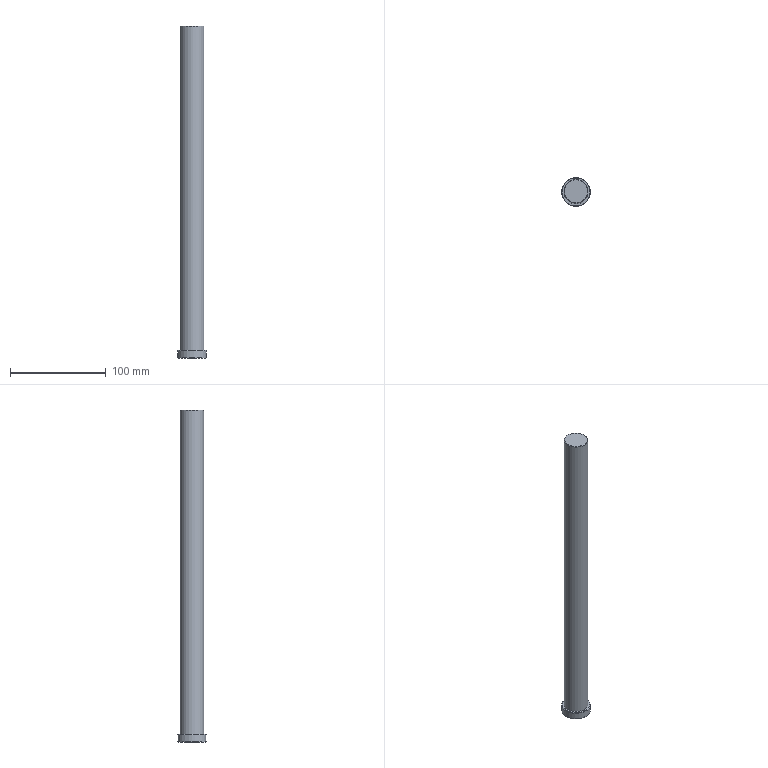Part | NX | features solid 2 | 1 solid | 8 faces | box 30 x 30 x 346 mm | volume 171537 mm3 | plane 3 | cone 3 | cylinder 2 | commonest cylinder face diameters 25 x1 30 x1
STEP:
#1=CARTESIAN_POINT('',(111.5,-195.,-337.5));
#2=VERTEX_POINT('',#1);
#3=CARTESIAN_POINT('',(99.,-195.,-337.5));
#4=DIRECTION('',(0.,0.,1.));
#5=DIRECTION('',(1.,0.,0.));
#6=AXIS2_PLACEMENT_3D('',#3,#4,#5);
#7=CIRCLE('',#6,12.5);
#8=EDGE_CURVE('',#2,#2,#7,.T.);
#9=ORIENTED_EDGE('',*,*,#8,.F.);
#10=EDGE_LOOP('',(#9));
#11=FACE_BOUND('',#10,.T.);
#12=CARTESIAN_POINT('',(113.5,-195.,-337.5));
#13=VERTEX_POINT('',#12);
#14=CARTESIAN_POINT('',(99.,-195.,-337.5));
#15=DIRECTION('',(0.,0.,1.));
#16=DIRECTION('',(1.,0.,0.));
#17=AXIS2_PLACEMENT_3D('',#14,#15,#16);
#18=CIRCLE('',#17,14.5);
#19=EDGE_CURVE('',#13,#13,#18,.T.);
#20=ORIENTED_EDGE('',*,*,#19,.T.);
#21=EDGE_LOOP('',(#20));
#22=FACE_BOUND('',#21,.T.);
#23=CARTESIAN_POINT('',(99.,-195.,-337.5));
#24=DIRECTION('',(0.,0.,1.));
#25=DIRECTION('',(1.,0.,0.));
#26=AXIS2_PLACEMENT_3D('',#23,#24,#25);
#27=PLANE('',#26);
#28=ADVANCED_FACE('',(#11,#22),#27,.T.);
#29=CARTESIAN_POINT('',(84.5,-195.,-345.5));
#30=VERTEX_POINT('',#29);
#31=CARTESIAN_POINT('',(99.,-195.,-345.5));
#32=DIRECTION('',(0.,0.,-1.));
#33=DIRECTION('',(-1.,0.,0.));
#34=AXIS2_PLACEMENT_3D('',#31,#32,#33);
#35=CIRCLE('',#34,14.5);
#36=EDGE_CURVE('',#30,#30,#35,.T.);
#37=ORIENTED_EDGE('',*,*,#36,.T.);
#38=EDGE_LOOP('',(#37));
#39=FACE_BOUND('',#38,.T.);
#40=CARTESIAN_POINT('',(99.,-195.,-345.5));
#41=DIRECTION('',(0.,0.,-1.));
#42=DIRECTION('',(-1.,0.,0.));
#43=AXIS2_PLACEMENT_3D('',#40,#41,#42);
#44=PLANE('',#43);
#45=ADVANCED_FACE('',(#39),#44,.T.);
#46=CARTESIAN_POINT('',(84.,-195.,-345.));
#47=VERTEX_POINT('',#46);
#48=CARTESIAN_POINT('',(99.,-195.,-345.));
#49=DIRECTION('',(0.,0.,-1.));
#50=DIRECTION('',(-1.,0.,0.));
#51=AXIS2_PLACEMENT_3D('',#48,#49,#50);
#52=CIRCLE('',#51,15.);
#53=EDGE_CURVE('',#47,#47,#52,.F.);
#54=ORIENTED_EDGE('',*,*,#53,.T.);
#55=EDGE_LOOP('',(#54));
#56=FACE_BOUND('',#55,.T.);
#57=CARTESIAN_POINT('',(114.,-195.,-338.));
#58=VERTEX_POINT('',#57);
#59=CARTESIAN_POINT('',(99.,-195.,-338.));
#60=DIRECTION('',(0.,0.,1.));
#61=DIRECTION('',(1.,0.,0.));
#62=AXIS2_PLACEMENT_3D('',#59,#60,#61);
#63=CIRCLE('',#62,15.);
#64=EDGE_CURVE('',#58,#58,#63,.F.);
#65=ORIENTED_EDGE('',*,*,#64,.T.);
#66=EDGE_LOOP('',(#65));
#67=FACE_BOUND('',#66,.T.);
#68=CARTESIAN_POINT('',(99.,-195.,-345.5));
#69=DIRECTION('',(0.,0.,1.));
#70=DIRECTION('',(1.,0.,0.));
#71=AXIS2_PLACEMENT_3D('',#68,#69,#70);
#72=CYLINDRICAL_SURFACE('',#71,15.);
#73=ADVANCED_FACE('',(#56,#67),#72,.T.);
#74=ORIENTED_EDGE('',*,*,#36,.F.);
#75=EDGE_LOOP('',(#74));
#76=FACE_BOUND('',#75,.T.);
#77=ORIENTED_EDGE('',*,*,#53,.F.);
#78=EDGE_LOOP('',(#77));
#79=FACE_BOUND('',#78,.T.);
#80=CARTESIAN_POINT('',(99.,-195.,-345.));
#81=DIRECTION('',(0.,0.,1.));
#82=DIRECTION('',(1.,0.,0.));
#83=AXIS2_PLACEMENT_3D('',#80,#81,#82);
#84=CONICAL_SURFACE('',#83,15.,0.7854);
#85=ADVANCED_FACE('',(#76,#79),#84,.T.);
#86=ORIENTED_EDGE('',*,*,#19,.F.);
#87=EDGE_LOOP('',(#86));
#88=FACE_BOUND('',#87,.T.);
#89=ORIENTED_EDGE('',*,*,#64,.F.);
#90=EDGE_LOOP('',(#89));
#91=FACE_BOUND('',#90,.T.);
#92=CARTESIAN_POINT('',(99.,-195.,-338.));
#93=DIRECTION('',(0.,0.,-1.));
#94=DIRECTION('',(-1.,0.,0.));
#95=AXIS2_PLACEMENT_3D('',#92,#93,#94);
#96=CONICAL_SURFACE('',#95,15.,0.7854);
#97=ADVANCED_FACE('',(#88,#91),#96,.T.);
#98=CARTESIAN_POINT('',(111.,-195.,0.5));
#99=VERTEX_POINT('',#98);
#100=CARTESIAN_POINT('',(99.,-195.,0.5));
#101=DIRECTION('',(0.,0.,1.));
#102=DIRECTION('',(1.,0.,0.));
#103=AXIS2_PLACEMENT_3D('',#100,#101,#102);
#104=CIRCLE('',#103,12.);
#105=EDGE_CURVE('',#99,#99,#104,.T.);
#106=ORIENTED_EDGE('',*,*,#105,.T.);
#107=EDGE_LOOP('',(#106));
#108=FACE_BOUND('',#107,.T.);
#109=CARTESIAN_POINT('',(99.,-195.,0.5));
#110=DIRECTION('',(0.,0.,1.));
#111=DIRECTION('',(1.,0.,0.));
#112=AXIS2_PLACEMENT_3D('',#109,#110,#111);
#113=PLANE('',#112);
#114=ADVANCED_FACE('',(#108),#113,.T.);
#115=ORIENTED_EDGE('',*,*,#8,.T.);
#116=EDGE_LOOP('',(#115));
#117=FACE_BOUND('',#116,.T.);
#118=CARTESIAN_POINT('',(111.5,-195.,0.));
#119=VERTEX_POINT('',#118);
#120=CARTESIAN_POINT('',(99.,-195.,0.));
#121=DIRECTION('',(0.,0.,1.));
#122=DIRECTION('',(1.,0.,0.));
#123=AXIS2_PLACEMENT_3D('',#120,#121,#122);
#124=CIRCLE('',#123,12.5);
#125=EDGE_CURVE('',#119,#119,#124,.F.);
#126=ORIENTED_EDGE('',*,*,#125,.T.);
#127=EDGE_LOOP('',(#126));
#128=FACE_BOUND('',#127,.T.);
#129=CARTESIAN_POINT('',(99.,-195.,-345.5));
#130=DIRECTION('',(0.,0.,1.));
#131=DIRECTION('',(1.,0.,0.));
#132=AXIS2_PLACEMENT_3D('',#129,#130,#131);
#133=CYLINDRICAL_SURFACE('',#132,12.5);
#134=ADVANCED_FACE('',(#117,#128),#133,.T.);
#135=ORIENTED_EDGE('',*,*,#105,.F.);
#136=EDGE_LOOP('',(#135));
#137=FACE_BOUND('',#136,.T.);
#138=ORIENTED_EDGE('',*,*,#125,.F.);
#139=EDGE_LOOP('',(#138));
#140=FACE_BOUND('',#139,.T.);
#141=CARTESIAN_POINT('',(99.,-195.,0.));
#142=DIRECTION('',(0.,0.,-1.));
#143=DIRECTION('',(-1.,0.,0.));
#144=AXIS2_PLACEMENT_3D('',#141,#142,#143);
#145=CONICAL_SURFACE('',#144,12.5,0.7854);
#146=ADVANCED_FACE('',(#137,#140),#145,.T.);
#147=CLOSED_SHELL('',(#28,#45,#73,#85,#97,#114,#134,#146));
#148=MANIFOLD_SOLID_BREP('',#147);
#149=(LENGTH_UNIT()NAMED_UNIT(*)SI_UNIT(.MILLI.,.METRE.));
#150=UNCERTAINTY_MEASURE_WITH_UNIT(LENGTH_MEASURE(0.00001),#149,'','');
#151=(NAMED_UNIT(*)PLANE_ANGLE_UNIT()SI_UNIT($,.RADIAN.));
#152=(NAMED_UNIT(*)SI_UNIT($,.STERADIAN.)SOLID_ANGLE_UNIT());
#153=(GEOMETRIC_REPRESENTATION_CONTEXT(3)GLOBAL_UNCERTAINTY_ASSIGNED_CONTEXT((#150))GLOBAL_UNIT_ASSIGNED_CONTEXT((#149,#151,#152))REPRESENTATION_CONTEXT('',''));
#154=ADVANCED_BREP_SHAPE_REPRESENTATION('',(#148),#153);